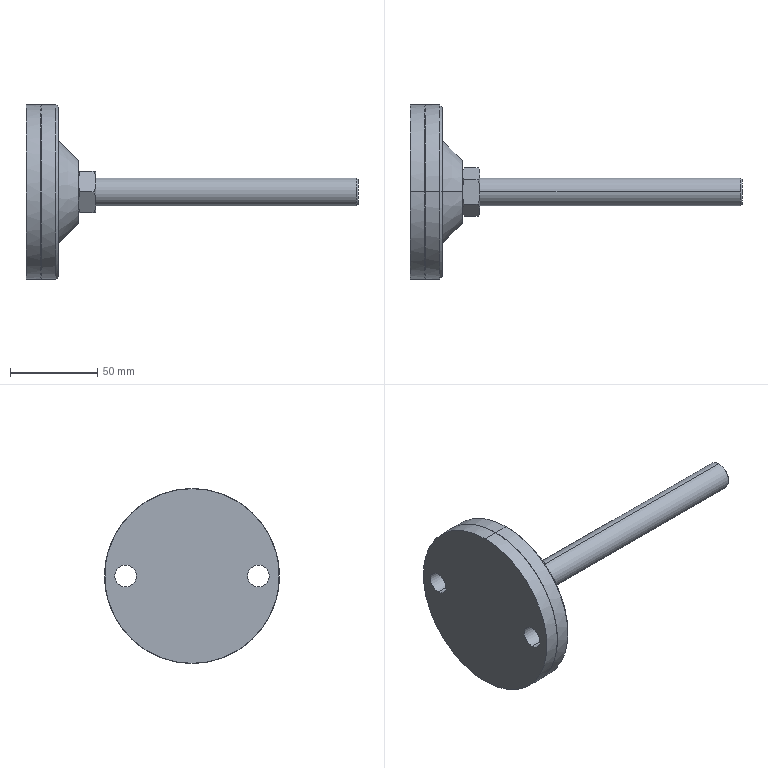Part | STEP file | C-CPVCH16-150 | 1 solid | 34 faces | box 190 x 100 x 100 mm | volume 196270 mm3 | plane 12 | cylinder 10 | cone 8 | spline 4 | commonest cylinder face diameters 12.5 x4 100 x4 16 x2
STEP:
#1=CARTESIAN_POINT('',(31.,-6.928,12.));
#2=VERTEX_POINT('',#1);
#3=CARTESIAN_POINT('',(30.133,0.,12.));
#4=VERTEX_POINT('',#3);
#5=CARTESIAN_POINT('',(31.,-6.928,12.));
#6=CARTESIAN_POINT('',(30.792,-6.375,12.));
#7=CARTESIAN_POINT('',(30.643,-5.81,12.));
#8=CARTESIAN_POINT('',(30.414,-4.667,12.));
#9=CARTESIAN_POINT('',(30.335,-4.089,12.));
#10=CARTESIAN_POINT('',(30.221,-2.923,12.));
#11=CARTESIAN_POINT('',(30.186,-2.337,12.));
#12=CARTESIAN_POINT('',(30.142,-1.168,12.));
#13=CARTESIAN_POINT('',(30.133,-0.5839,12.));
#14=CARTESIAN_POINT('',(30.133,0.,12.));
#15=B_SPLINE_CURVE_WITH_KNOTS('',3,(#5,#6,#7,#8,#9,#10,#11,#12,#13,#14),.UNSPECIFIED.,.F.,.F.,(4,2,2,2,4),(0.,0.001749,0.003497,0.005246,0.006994),.UNSPECIFIED.);
#16=EDGE_CURVE('',#2,#4,#15,.T.);
#17=ORIENTED_EDGE('',*,*,#16,.T.);
#18=CARTESIAN_POINT('',(30.,0.,10.856));
#19=VERTEX_POINT('',#18);
#20=CARTESIAN_POINT('',(35.,0.,10.856));
#21=DIRECTION('',(0.,-1.,0.));
#22=DIRECTION('',(0.,0.,1.));
#23=AXIS2_PLACEMENT_3D('',#20,#21,#22);
#24=CIRCLE('',#23,5.);
#25=EDGE_CURVE('',#4,#19,#24,.T.);
#26=ORIENTED_EDGE('',*,*,#25,.T.);
#27=CARTESIAN_POINT('',(30.,0.,-10.856));
#28=VERTEX_POINT('',#27);
#29=CARTESIAN_POINT('',(30.,0.,10.856));
#30=CARTESIAN_POINT('',(30.,-21.713,10.856));
#31=CARTESIAN_POINT('',(30.,-21.713,-10.856));
#32=CARTESIAN_POINT('',(30.,0.,-10.856));
#33=(BOUNDED_CURVE()B_SPLINE_CURVE(3,(#29,#30,#31,#32),.UNSPECIFIED.,.F.,.T.)B_SPLINE_CURVE_WITH_KNOTS((4,4),(0.5,1.),.UNSPECIFIED.)CURVE()GEOMETRIC_REPRESENTATION_ITEM()RATIONAL_B_SPLINE_CURVE((1.,0.3333,0.3333,1.))REPRESENTATION_ITEM(''));
#34=EDGE_CURVE('',#19,#28,#33,.T.);
#35=ORIENTED_EDGE('',*,*,#34,.T.);
#36=CARTESIAN_POINT('',(30.133,0.,-12.));
#37=VERTEX_POINT('',#36);
#38=CARTESIAN_POINT('',(35.,0.,-10.856));
#39=DIRECTION('',(0.,1.,0.));
#40=DIRECTION('',(0.,0.,-1.));
#41=AXIS2_PLACEMENT_3D('',#38,#39,#40);
#42=CIRCLE('',#41,5.);
#43=EDGE_CURVE('',#37,#28,#42,.T.);
#44=ORIENTED_EDGE('',*,*,#43,.F.);
#45=CARTESIAN_POINT('',(31.,-6.928,-12.));
#46=VERTEX_POINT('',#45);
#47=CARTESIAN_POINT('',(30.133,0.,-12.));
#48=CARTESIAN_POINT('',(30.133,-0.583,-12.));
#49=CARTESIAN_POINT('',(30.142,-1.166,-12.));
#50=CARTESIAN_POINT('',(30.186,-2.33,-12.));
#51=CARTESIAN_POINT('',(30.221,-2.912,-12.));
#52=CARTESIAN_POINT('',(30.334,-4.075,-12.));
#53=CARTESIAN_POINT('',(30.413,-4.659,-12.));
#54=CARTESIAN_POINT('',(30.643,-5.81,-12.));
#55=CARTESIAN_POINT('',(30.793,-6.376,-12.));
#56=CARTESIAN_POINT('',(31.,-6.928,-12.));
#57=B_SPLINE_CURVE_WITH_KNOTS('',3,(#47,#48,#49,#50,#51,#52,#53,#54,#55,#56),.UNSPECIFIED.,.F.,.F.,(4,2,2,2,4),(0.006994,0.00874,0.01049,0.01223,0.01398),.UNSPECIFIED.);
#58=EDGE_CURVE('',#37,#46,#57,.T.);
#59=ORIENTED_EDGE('',*,*,#58,.T.);
#60=CARTESIAN_POINT('',(31.,-13.856,0.));
#61=VERTEX_POINT('',#60);
#62=CARTESIAN_POINT('',(31.,-6.928,-12.));
#63=CARTESIAN_POINT('',(30.793,-7.205,-11.521));
#64=CARTESIAN_POINT('',(30.643,-7.487,-11.032));
#65=CARTESIAN_POINT('',(30.414,-8.058,-10.043));
#66=CARTESIAN_POINT('',(30.336,-8.347,-9.543));
#67=CARTESIAN_POINT('',(30.222,-8.929,-8.534));
#68=CARTESIAN_POINT('',(30.187,-9.222,-8.027));
#69=CARTESIAN_POINT('',(30.142,-9.806,-7.015));
#70=CARTESIAN_POINT('',(30.133,-10.098,-6.51));
#71=CARTESIAN_POINT('',(30.132,-10.681,-5.499));
#72=CARTESIAN_POINT('',(30.142,-10.973,-4.994));
#73=CARTESIAN_POINT('',(30.186,-11.556,-3.985));
#74=CARTESIAN_POINT('',(30.221,-11.847,-3.48));
#75=CARTESIAN_POINT('',(30.333,-12.429,-2.473));
#76=CARTESIAN_POINT('',(30.412,-12.721,-1.967));
#77=CARTESIAN_POINT('',(30.642,-13.297,-0.9692));
#78=CARTESIAN_POINT('',(30.793,-13.58,-0.4783));
#79=CARTESIAN_POINT('',(31.,-13.856,0.));
#80=B_SPLINE_CURVE_WITH_KNOTS('',3,(#62,#63,#64,#65,#66,#67,#68,#69,#70,#71,#72,#73,#74,#75,#76,#77,#78,#79),.UNSPECIFIED.,.F.,.F.,(4,2,2,2,2,2,2,2,4),(0.,0.001747,0.003494,0.005242,0.006989,0.008736,0.01048,0.01223,0.01398),.UNSPECIFIED.);
#81=EDGE_CURVE('',#46,#61,#80,.T.);
#82=ORIENTED_EDGE('',*,*,#81,.T.);
#83=CARTESIAN_POINT('',(31.,-13.856,0.));
#84=CARTESIAN_POINT('',(30.793,-13.58,0.4789));
#85=CARTESIAN_POINT('',(30.643,-13.298,0.9675));
#86=CARTESIAN_POINT('',(30.414,-12.727,1.957));
#87=CARTESIAN_POINT('',(30.336,-12.438,2.457));
#88=CARTESIAN_POINT('',(30.222,-11.855,3.466));
#89=CARTESIAN_POINT('',(30.187,-11.563,3.973));
#90=CARTESIAN_POINT('',(30.142,-10.979,4.985));
#91=CARTESIAN_POINT('',(30.133,-10.687,5.49));
#92=CARTESIAN_POINT('',(30.132,-10.103,6.501));
#93=CARTESIAN_POINT('',(30.142,-9.812,7.006));
#94=CARTESIAN_POINT('',(30.186,-9.229,8.015));
#95=CARTESIAN_POINT('',(30.221,-8.938,8.52));
#96=CARTESIAN_POINT('',(30.333,-8.356,9.527));
#97=CARTESIAN_POINT('',(30.412,-8.064,10.033));
#98=CARTESIAN_POINT('',(30.642,-7.488,11.031));
#99=CARTESIAN_POINT('',(30.793,-7.204,11.522));
#100=CARTESIAN_POINT('',(31.,-6.928,12.));
#101=B_SPLINE_CURVE_WITH_KNOTS('',3,(#83,#84,#85,#86,#87,#88,#89,#90,#91,#92,#93,#94,#95,#96,#97,#98,#99,#100),.UNSPECIFIED.,.F.,.F.,(4,2,2,2,2,2,2,2,4),(0.,0.001747,0.003494,0.005242,0.006989,0.008736,0.01048,0.01223,0.01398),.UNSPECIFIED.);
#102=EDGE_CURVE('',#61,#2,#101,.T.);
#103=ORIENTED_EDGE('',*,*,#102,.T.);
#104=EDGE_LOOP('',(#17,#26,#35,#44,#59,#82,#103));
#105=FACE_OUTER_BOUND('',#104,.T.);
#106=CARTESIAN_POINT('',(31.012,0.,13.872));
#107=CARTESIAN_POINT('',(31.012,-27.744,13.872));
#108=CARTESIAN_POINT('',(31.012,-27.744,-13.872));
#109=CARTESIAN_POINT('',(31.012,0.,-13.872));
#110=CARTESIAN_POINT('',(30.349,0.,12.996));
#111=CARTESIAN_POINT('',(30.349,-25.992,12.996));
#112=CARTESIAN_POINT('',(30.349,-25.992,-12.996));
#113=CARTESIAN_POINT('',(30.349,0.,-12.996));
#114=CARTESIAN_POINT('',(30.,0.,11.955));
#115=CARTESIAN_POINT('',(30.,-23.909,11.955));
#116=CARTESIAN_POINT('',(30.,-23.909,-11.955));
#117=CARTESIAN_POINT('',(30.,0.,-11.955));
#118=CARTESIAN_POINT('',(30.,0.,10.856));
#119=CARTESIAN_POINT('',(30.,-21.713,10.856));
#120=CARTESIAN_POINT('',(30.,-21.713,-10.856));
#121=CARTESIAN_POINT('',(30.,0.,-10.856));
#122=(BOUNDED_SURFACE()B_SPLINE_SURFACE(3,3,((#106,#107,#108,#109),(#110,#111,#112,#113),(#114,#115,#116,#117),(#118,#119,#120,#121)),.UNSPECIFIED.,.F.,.F.,.F.)B_SPLINE_SURFACE_WITH_KNOTS((4,4),(4,4),(0.,1.),(0.,1.),.UNSPECIFIED.)GEOMETRIC_REPRESENTATION_ITEM()RATIONAL_B_SPLINE_SURFACE(((1.,0.3333,0.3333,1.),(0.9654,0.3218,0.3218,0.9654),(0.9654,0.3218,0.3218,0.9654),(1.,0.3333,0.3333,1.)))REPRESENTATION_ITEM('')SURFACE());
#123=ADVANCED_FACE('',(#105),#122,.T.);
#124=CARTESIAN_POINT('',(40.,0.,-10.856));
#125=VERTEX_POINT('',#124);
#126=CARTESIAN_POINT('',(40.,0.,10.856));
#127=VERTEX_POINT('',#126);
#128=CARTESIAN_POINT('',(40.,0.,-10.856));
#129=CARTESIAN_POINT('',(40.,-21.713,-10.856));
#130=CARTESIAN_POINT('',(40.,-21.713,10.856));
#131=CARTESIAN_POINT('',(40.,0.,10.856));
#132=(BOUNDED_CURVE()B_SPLINE_CURVE(3,(#128,#129,#130,#131),.UNSPECIFIED.,.F.,.F.)B_SPLINE_CURVE_WITH_KNOTS((4,4),(0.,0.5),.UNSPECIFIED.)CURVE()GEOMETRIC_REPRESENTATION_ITEM()RATIONAL_B_SPLINE_CURVE((1.,0.3333,0.3333,1.))REPRESENTATION_ITEM(''));
#133=EDGE_CURVE('',#125,#127,#132,.T.);
#134=ORIENTED_EDGE('',*,*,#133,.T.);
#135=CARTESIAN_POINT('',(39.867,0.,12.));
#136=VERTEX_POINT('',#135);
#137=CARTESIAN_POINT('',(35.,0.,10.856));
#138=DIRECTION('',(0.,-1.,0.));
#139=DIRECTION('',(0.,0.,1.));
#140=AXIS2_PLACEMENT_3D('',#137,#138,#139);
#141=CIRCLE('',#140,5.);
#142=EDGE_CURVE('',#127,#136,#141,.T.);
#143=ORIENTED_EDGE('',*,*,#142,.T.);
#144=CARTESIAN_POINT('',(39.,-6.928,12.));
#145=VERTEX_POINT('',#144);
#146=CARTESIAN_POINT('',(39.867,0.,12.));
#147=CARTESIAN_POINT('',(39.867,-0.583,12.));
#148=CARTESIAN_POINT('',(39.858,-1.166,12.));
#149=CARTESIAN_POINT('',(39.814,-2.33,12.));
#150=CARTESIAN_POINT('',(39.779,-2.912,12.));
#151=CARTESIAN_POINT('',(39.666,-4.075,12.));
#152=CARTESIAN_POINT('',(39.587,-4.659,12.));
#153=CARTESIAN_POINT('',(39.357,-5.81,12.));
#154=CARTESIAN_POINT('',(39.207,-6.376,12.));
#155=CARTESIAN_POINT('',(39.,-6.928,12.));
#156=B_SPLINE_CURVE_WITH_KNOTS('',3,(#146,#147,#148,#149,#150,#151,#152,#153,#154,#155),.UNSPECIFIED.,.F.,.F.,(4,2,2,2,4),(0.006994,0.00874,0.01049,0.01223,0.01398),.UNSPECIFIED.);
#157=EDGE_CURVE('',#136,#145,#156,.T.);
#158=ORIENTED_EDGE('',*,*,#157,.T.);
#159=CARTESIAN_POINT('',(39.,-13.856,0.));
#160=VERTEX_POINT('',#159);
#161=CARTESIAN_POINT('',(39.,-6.928,12.));
#162=CARTESIAN_POINT('',(39.207,-7.205,11.521));
#163=CARTESIAN_POINT('',(39.357,-7.487,11.032));
#164=CARTESIAN_POINT('',(39.586,-8.058,10.043));
#165=CARTESIAN_POINT('',(39.664,-8.347,9.543));
#166=CARTESIAN_POINT('',(39.778,-8.929,8.534));
#167=CARTESIAN_POINT('',(39.813,-9.222,8.027));
#168=CARTESIAN_POINT('',(39.858,-9.806,7.015));
#169=CARTESIAN_POINT('',(39.867,-10.098,6.51));
#170=CARTESIAN_POINT('',(39.868,-10.681,5.499));
#171=CARTESIAN_POINT('',(39.858,-10.973,4.994));
#172=CARTESIAN_POINT('',(39.814,-11.556,3.985));
#173=CARTESIAN_POINT('',(39.779,-11.847,3.48));
#174=CARTESIAN_POINT('',(39.667,-12.429,2.473));
#175=CARTESIAN_POINT('',(39.588,-12.721,1.967));
#176=CARTESIAN_POINT('',(39.358,-13.297,0.9692));
#177=CARTESIAN_POINT('',(39.207,-13.58,0.4783));
#178=CARTESIAN_POINT('',(39.,-13.856,0.));
#179=B_SPLINE_CURVE_WITH_KNOTS('',3,(#161,#162,#163,#164,#165,#166,#167,#168,#169,#170,#171,#172,#173,#174,#175,#176,#177,#178),.UNSPECIFIED.,.F.,.F.,(4,2,2,2,2,2,2,2,4),(0.,0.001747,0.003494,0.005242,0.006989,0.008736,0.01048,0.01223,0.01398),.UNSPECIFIED.);
#180=EDGE_CURVE('',#145,#160,#179,.T.);
#181=ORIENTED_EDGE('',*,*,#180,.T.);
#182=CARTESIAN_POINT('',(39.,-6.928,-12.));
#183=VERTEX_POINT('',#182);
#184=CARTESIAN_POINT('',(39.,-13.856,0.));
#185=CARTESIAN_POINT('',(39.207,-13.58,-0.4789));
#186=CARTESIAN_POINT('',(39.357,-13.298,-0.9675));
#187=CARTESIAN_POINT('',(39.586,-12.727,-1.957));
#188=CARTESIAN_POINT('',(39.664,-12.438,-2.457));
#189=CARTESIAN_POINT('',(39.778,-11.855,-3.466));
#190=CARTESIAN_POINT('',(39.813,-11.563,-3.973));
#191=CARTESIAN_POINT('',(39.858,-10.979,-4.985));
#192=CARTESIAN_POINT('',(39.867,-10.687,-5.49));
#193=CARTESIAN_POINT('',(39.868,-10.103,-6.501));
#194=CARTESIAN_POINT('',(39.858,-9.812,-7.006));
#195=CARTESIAN_POINT('',(39.814,-9.229,-8.015));
#196=CARTESIAN_POINT('',(39.779,-8.938,-8.52));
#197=CARTESIAN_POINT('',(39.667,-8.356,-9.527));
#198=CARTESIAN_POINT('',(39.588,-8.064,-10.033));
#199=CARTESIAN_POINT('',(39.358,-7.488,-11.031));
#200=CARTESIAN_POINT('',(39.207,-7.204,-11.522));
#201=CARTESIAN_POINT('',(39.,-6.928,-12.));
#202=B_SPLINE_CURVE_WITH_KNOTS('',3,(#184,#185,#186,#187,#188,#189,#190,#191,#192,#193,#194,#195,#196,#197,#198,#199,#200,#201),.UNSPECIFIED.,.F.,.F.,(4,2,2,2,2,2,2,2,4),(0.,0.001747,0.003494,0.005242,0.006989,0.008736,0.01048,0.01223,0.01398),.UNSPECIFIED.);
#203=EDGE_CURVE('',#160,#183,#202,.T.);
#204=ORIENTED_EDGE('',*,*,#203,.T.);
#205=CARTESIAN_POINT('',(39.867,0.,-12.));
#206=VERTEX_POINT('',#205);
#207=CARTESIAN_POINT('',(39.,-6.928,-12.));
#208=CARTESIAN_POINT('',(39.208,-6.375,-12.));
#209=CARTESIAN_POINT('',(39.357,-5.81,-12.));
#210=CARTESIAN_POINT('',(39.586,-4.667,-12.));
#211=CARTESIAN_POINT('',(39.665,-4.089,-12.));
#212=CARTESIAN_POINT('',(39.779,-2.923,-12.));
#213=CARTESIAN_POINT('',(39.814,-2.337,-12.));
#214=CARTESIAN_POINT('',(39.858,-1.168,-12.));
#215=CARTESIAN_POINT('',(39.867,-0.5839,-12.));
#216=CARTESIAN_POINT('',(39.867,0.,-12.));
#217=B_SPLINE_CURVE_WITH_KNOTS('',3,(#207,#208,#209,#210,#211,#212,#213,#214,#215,#216),.UNSPECIFIED.,.F.,.F.,(4,2,2,2,4),(0.,0.001749,0.003497,0.005246,0.006994),.UNSPECIFIED.);
#218=EDGE_CURVE('',#183,#206,#217,.T.);
#219=ORIENTED_EDGE('',*,*,#218,.T.);
#220=CARTESIAN_POINT('',(35.,0.,-10.856));
#221=DIRECTION('',(0.,1.,0.));
#222=DIRECTION('',(0.,0.,-1.));
#223=AXIS2_PLACEMENT_3D('',#220,#221,#222);
#224=CIRCLE('',#223,5.);
#225=EDGE_CURVE('',#125,#206,#224,.T.);
#226=ORIENTED_EDGE('',*,*,#225,.F.);
#227=EDGE_LOOP('',(#134,#143,#158,#181,#204,#219,#226));
#228=FACE_OUTER_BOUND('',#227,.T.);
#229=CARTESIAN_POINT('',(40.,0.,10.856));
#230=CARTESIAN_POINT('',(40.,-21.713,10.856));
#231=CARTESIAN_POINT('',(40.,-21.713,-10.856));
#232=CARTESIAN_POINT('',(40.,0.,-10.856));
#233=CARTESIAN_POINT('',(40.,0.,11.955));
#234=CARTESIAN_POINT('',(40.,-23.909,11.955));
#235=CARTESIAN_POINT('',(40.,-23.909,-11.955));
#236=CARTESIAN_POINT('',(40.,0.,-11.955));
#237=CARTESIAN_POINT('',(39.651,0.,12.996));
#238=CARTESIAN_POINT('',(39.651,-25.992,12.996));
#239=CARTESIAN_POINT('',(39.651,-25.992,-12.996));
#240=CARTESIAN_POINT('',(39.651,0.,-12.996));
#241=CARTESIAN_POINT('',(38.988,0.,13.872));
#242=CARTESIAN_POINT('',(38.988,-27.744,13.872));
#243=CARTESIAN_POINT('',(38.988,-27.744,-13.872));
#244=CARTESIAN_POINT('',(38.988,0.,-13.872));
#245=(BOUNDED_SURFACE()B_SPLINE_SURFACE(3,3,((#229,#230,#231,#232),(#233,#234,#235,#236),(#237,#238,#239,#240),(#241,#242,#243,#244)),.UNSPECIFIED.,.F.,.F.,.F.)B_SPLINE_SURFACE_WITH_KNOTS((4,4),(4,4),(0.,1.),(0.,1.),.UNSPECIFIED.)GEOMETRIC_REPRESENTATION_ITEM()RATIONAL_B_SPLINE_SURFACE(((1.,0.3333,0.3333,1.),(0.9654,0.3218,0.3218,0.9654),(0.9654,0.3218,0.3218,0.9654),(1.,0.3333,0.3333,1.)))REPRESENTATION_ITEM('')SURFACE());
#246=ADVANCED_FACE('',(#228),#245,.T.);
#247=CARTESIAN_POINT('',(18.5,-38.,-6.25));
#248=VERTEX_POINT('',#247);
#249=CARTESIAN_POINT('',(18.5,-38.,6.25));
#250=VERTEX_POINT('',#249);
#251=CARTESIAN_POINT('',(18.5,-38.,0.));
#252=DIRECTION('',(-1.,0.,0.));
#253=DIRECTION('',(0.,0.,1.));
#254=AXIS2_PLACEMENT_3D('',#251,#252,#253);
#255=CIRCLE('',#254,6.25);
#256=EDGE_CURVE('',#248,#250,#255,.T.);
#257=ORIENTED_EDGE('',*,*,#256,.F.);
#258=CARTESIAN_POINT('',(0.,-38.,-6.25));
#259=VERTEX_POINT('',#258);
#260=CARTESIAN_POINT('',(18.5,-38.,-6.25));
#261=DIRECTION('',(-1.,0.,0.));
#262=VECTOR('',#261,1000.);
#263=LINE('',#260,#262);
#264=EDGE_CURVE('',#248,#259,#263,.T.);
#265=ORIENTED_EDGE('',*,*,#264,.T.);
#266=CARTESIAN_POINT('',(0.,-38.,6.25));
#267=VERTEX_POINT('',#266);
#268=CARTESIAN_POINT('',(0.,-38.,0.));
#269=DIRECTION('',(-1.,0.,0.));
#270=DIRECTION('',(0.,0.,1.));
#271=AXIS2_PLACEMENT_3D('',#268,#269,#270);
#272=CIRCLE('',#271,6.25);
#273=EDGE_CURVE('',#259,#267,#272,.T.);
#274=ORIENTED_EDGE('',*,*,#273,.T.);
#275=CARTESIAN_POINT('',(18.5,-38.,6.25));
#276=DIRECTION('',(-1.,0.,0.));
#277=VECTOR('',#276,1000.);
#278=LINE('',#275,#277);
#279=EDGE_CURVE('',#250,#267,#278,.T.);
#280=ORIENTED_EDGE('',*,*,#279,.F.);
#281=EDGE_LOOP('',(#257,#265,#274,#280));
#282=FACE_OUTER_BOUND('',#281,.T.);
#283=CARTESIAN_POINT('',(18.5,-38.,0.));
#284=DIRECTION('',(-1.,0.,0.));
#285=DIRECTION('',(0.,0.,1.));
#286=AXIS2_PLACEMENT_3D('',#283,#284,#285);
#287=CYLINDRICAL_SURFACE('',#286,6.25);
#288=ADVANCED_FACE('',(#282),#287,.F.);
#289=CARTESIAN_POINT('',(18.5,38.,-6.25));
#290=VERTEX_POINT('',#289);
#291=CARTESIAN_POINT('',(18.5,38.,6.25));
#292=VERTEX_POINT('',#291);
#293=CARTESIAN_POINT('',(18.5,38.,0.));
#294=DIRECTION('',(-1.,0.,0.));
#295=DIRECTION('',(0.,0.,1.));
#296=AXIS2_PLACEMENT_3D('',#293,#294,#295);
#297=CIRCLE('',#296,6.25);
#298=EDGE_CURVE('',#290,#292,#297,.T.);
#299=ORIENTED_EDGE('',*,*,#298,.F.);
#300=CARTESIAN_POINT('',(0.,38.,-6.25));
#301=VERTEX_POINT('',#300);
#302=CARTESIAN_POINT('',(18.5,38.,-6.25));
#303=DIRECTION('',(-1.,0.,0.));
#304=VECTOR('',#303,1000.);
#305=LINE('',#302,#304);
#306=EDGE_CURVE('',#290,#301,#305,.T.);
#307=ORIENTED_EDGE('',*,*,#306,.T.);
#308=CARTESIAN_POINT('',(0.,38.,6.25));
#309=VERTEX_POINT('',#308);
#310=CARTESIAN_POINT('',(0.,38.,0.));
#311=DIRECTION('',(-1.,0.,0.));
#312=DIRECTION('',(0.,0.,1.));
#313=AXIS2_PLACEMENT_3D('',#310,#311,#312);
#314=CIRCLE('',#313,6.25);
#315=EDGE_CURVE('',#301,#309,#314,.T.);
#316=ORIENTED_EDGE('',*,*,#315,.T.);
#317=CARTESIAN_POINT('',(18.5,38.,6.25));
#318=DIRECTION('',(-1.,0.,0.));
#319=VECTOR('',#318,1000.);
#320=LINE('',#317,#319);
#321=EDGE_CURVE('',#292,#309,#320,.T.);
#322=ORIENTED_EDGE('',*,*,#321,.F.);
#323=EDGE_LOOP('',(#299,#307,#316,#322));
#324=FACE_OUTER_BOUND('',#323,.T.);
#325=CARTESIAN_POINT('',(18.5,38.,0.));
#326=DIRECTION('',(-1.,0.,0.));
#327=DIRECTION('',(0.,0.,1.));
#328=AXIS2_PLACEMENT_3D('',#325,#326,#327);
#329=CYLINDRICAL_SURFACE('',#328,6.25);
#330=ADVANCED_FACE('',(#324),#329,.F.);
#331=CARTESIAN_POINT('',(8.5,0.,50.));
#332=VERTEX_POINT('',#331);
#333=CARTESIAN_POINT('',(8.5,0.,-50.));
#334=VERTEX_POINT('',#333);
#335=CARTESIAN_POINT('',(8.5,0.,0.));
#336=DIRECTION('',(-1.,0.,0.));
#337=DIRECTION('',(0.,0.,1.));
#338=AXIS2_PLACEMENT_3D('',#335,#336,#337);
#339=CIRCLE('',#338,50.);
#340=EDGE_CURVE('',#332,#334,#339,.T.);
#341=ORIENTED_EDGE('',*,*,#340,.T.);
#342=CARTESIAN_POINT('',(0.,0.,-50.));
#343=VERTEX_POINT('',#342);
#344=CARTESIAN_POINT('',(190.,0.,-50.));
#345=DIRECTION('',(-1.,0.,0.));
#346=VECTOR('',#345,1000.);
#347=LINE('',#344,#346);
#348=EDGE_CURVE('',#334,#343,#347,.T.);
#349=ORIENTED_EDGE('',*,*,#348,.T.);
#350=CARTESIAN_POINT('',(0.,0.,50.));
#351=VERTEX_POINT('',#350);
#352=CARTESIAN_POINT('',(0.,0.,0.));
#353=DIRECTION('',(1.,0.,0.));
#354=DIRECTION('',(0.,0.,1.));
#355=AXIS2_PLACEMENT_3D('',#352,#353,#354);
#356=CIRCLE('',#355,50.);
#357=EDGE_CURVE('',#343,#351,#356,.T.);
#358=ORIENTED_EDGE('',*,*,#357,.T.);
#359=CARTESIAN_POINT('',(190.,0.,50.));
#360=DIRECTION('',(-1.,0.,0.));
#361=VECTOR('',#360,1000.);
#362=LINE('',#359,#361);
#363=EDGE_CURVE('',#332,#351,#362,.T.);
#364=ORIENTED_EDGE('',*,*,#363,.F.);
#365=EDGE_LOOP('',(#341,#349,#358,#364));
#366=FACE_OUTER_BOUND('',#365,.T.);
#367=CARTESIAN_POINT('',(190.,0.,0.));
#368=DIRECTION('',(-1.,0.,0.));
#369=DIRECTION('',(0.,0.,1.));
#370=AXIS2_PLACEMENT_3D('',#367,#368,#369);
#371=CYLINDRICAL_SURFACE('',#370,50.);
#372=ADVANCED_FACE('',(#366),#371,.T.);
#373=CARTESIAN_POINT('',(18.5,0.,48.5));
#374=VERTEX_POINT('',#373);
#375=CARTESIAN_POINT('',(18.5,0.,-48.5));
#376=VERTEX_POINT('',#375);
#377=CARTESIAN_POINT('',(18.5,0.,0.));
#378=DIRECTION('',(-1.,0.,0.));
#379=DIRECTION('',(0.,0.,1.));
#380=AXIS2_PLACEMENT_3D('',#377,#378,#379);
#381=CIRCLE('',#380,48.5);
#382=EDGE_CURVE('',#374,#376,#381,.T.);
#383=ORIENTED_EDGE('',*,*,#382,.T.);
#384=CARTESIAN_POINT('',(17.,0.,-50.));
#385=VERTEX_POINT('',#384);
#386=CARTESIAN_POINT('',(17.,0.,-50.));
#387=DIRECTION('',(-0.7071,0.,-0.7071));
#388=VECTOR('',#387,1000.);
#389=LINE('',#386,#388);
#390=EDGE_CURVE('',#376,#385,#389,.T.);
#391=ORIENTED_EDGE('',*,*,#390,.T.);
#392=CARTESIAN_POINT('',(17.,0.,50.));
#393=VERTEX_POINT('',#392);
#394=CARTESIAN_POINT('',(17.,0.,0.));
#395=DIRECTION('',(1.,0.,0.));
#396=DIRECTION('',(0.,0.,1.));
#397=AXIS2_PLACEMENT_3D('',#394,#395,#396);
#398=CIRCLE('',#397,50.);
#399=EDGE_CURVE('',#385,#393,#398,.T.);
#400=ORIENTED_EDGE('',*,*,#399,.T.);
#401=CARTESIAN_POINT('',(17.,0.,50.));
#402=DIRECTION('',(-0.7071,0.,0.7071));
#403=VECTOR('',#402,1000.);
#404=LINE('',#401,#403);
#405=EDGE_CURVE('',#374,#393,#404,.T.);
#406=ORIENTED_EDGE('',*,*,#405,.F.);
#407=EDGE_LOOP('',(#383,#391,#400,#406));
#408=FACE_OUTER_BOUND('',#407,.T.);
#409=CARTESIAN_POINT('',(17.,0.,0.));
#410=DIRECTION('',(-1.,0.,0.));
#411=DIRECTION('',(0.,0.,1.));
#412=AXIS2_PLACEMENT_3D('',#409,#410,#411);
#413=CONICAL_SURFACE('',#412,50.,0.7854);
#414=ADVANCED_FACE('',(#408),#413,.T.);
#415=CARTESIAN_POINT('',(30.,0.,18.));
#416=VERTEX_POINT('',#415);
#417=CARTESIAN_POINT('',(30.,0.,-18.));
#418=VERTEX_POINT('',#417);
#419=CARTESIAN_POINT('',(30.,0.,0.));
#420=DIRECTION('',(-1.,0.,0.));
#421=DIRECTION('',(0.,0.,1.));
#422=AXIS2_PLACEMENT_3D('',#419,#420,#421);
#423=CIRCLE('',#422,18.);
#424=EDGE_CURVE('',#416,#418,#423,.T.);
#425=ORIENTED_EDGE('',*,*,#424,.T.);
#426=CARTESIAN_POINT('',(18.5,0.,-29.5));
#427=VERTEX_POINT('',#426);
#428=CARTESIAN_POINT('',(18.5,0.,-29.5));
#429=DIRECTION('',(-0.7071,0.,-0.7071));
#430=VECTOR('',#429,1000.);
#431=LINE('',#428,#430);
#432=EDGE_CURVE('',#418,#427,#431,.T.);
#433=ORIENTED_EDGE('',*,*,#432,.T.);
#434=CARTESIAN_POINT('',(18.5,0.,29.5));
#435=VERTEX_POINT('',#434);
#436=CARTESIAN_POINT('',(18.5,0.,0.));
#437=DIRECTION('',(1.,0.,0.));
#438=DIRECTION('',(0.,0.,1.));
#439=AXIS2_PLACEMENT_3D('',#436,#437,#438);
#440=CIRCLE('',#439,29.5);
#441=EDGE_CURVE('',#427,#435,#440,.T.);
#442=ORIENTED_EDGE('',*,*,#441,.T.);
#443=CARTESIAN_POINT('',(18.5,0.,29.5));
#444=DIRECTION('',(-0.7071,0.,0.7071));
#445=VECTOR('',#444,1000.);
#446=LINE('',#443,#445);
#447=EDGE_CURVE('',#416,#435,#446,.T.);
#448=ORIENTED_EDGE('',*,*,#447,.F.);
#449=EDGE_LOOP('',(#425,#433,#442,#448));
#450=FACE_OUTER_BOUND('',#449,.T.);
#451=CARTESIAN_POINT('',(18.5,0.,0.));
#452=DIRECTION('',(-1.,0.,0.));
#453=DIRECTION('',(0.,0.,1.));
#454=AXIS2_PLACEMENT_3D('',#451,#452,#453);
#455=CONICAL_SURFACE('',#454,29.5,0.7854);
#456=ADVANCED_FACE('',(#450),#455,.T.);
#457=CARTESIAN_POINT('',(8.5,49.9,0.));
#458=VERTEX_POINT('',#457);
#459=CARTESIAN_POINT('',(8.5,-49.9,0.));
#460=VERTEX_POINT('',#459);
#461=CARTESIAN_POINT('',(8.5,0.,0.));
#462=DIRECTION('',(1.,0.,0.));
#463=DIRECTION('',(0.,1.,0.));
#464=AXIS2_PLACEMENT_3D('',#461,#462,#463);
#465=CIRCLE('',#464,49.9);
#466=EDGE_CURVE('',#458,#460,#465,.T.);
#467=ORIENTED_EDGE('',*,*,#466,.T.);
#468=CARTESIAN_POINT('',(8.6,-50.,0.));
#469=VERTEX_POINT('',#468);
#470=CARTESIAN_POINT('',(8.6,-50.,0.));
#471=DIRECTION('',(0.7071,-0.7071,0.));
#472=VECTOR('',#471,1000.);
#473=LINE('',#470,#472);
#474=EDGE_CURVE('',#460,#469,#473,.T.);
#475=ORIENTED_EDGE('',*,*,#474,.T.);
#476=CARTESIAN_POINT('',(8.6,0.,50.));
#477=VERTEX_POINT('',#476);
#478=CARTESIAN_POINT('',(8.6,0.,0.));
#479=DIRECTION('',(-1.,0.,0.));
#480=DIRECTION('',(0.,0.,-1.));
#481=AXIS2_PLACEMENT_3D('',#478,#479,#480);
#482=CIRCLE('',#481,50.);
#483=EDGE_CURVE('',#469,#477,#482,.T.);
#484=ORIENTED_EDGE('',*,*,#483,.T.);
#485=CARTESIAN_POINT('',(8.6,50.,0.));
#486=VERTEX_POINT('',#485);
#487=CARTESIAN_POINT('',(8.6,0.,0.));
#488=DIRECTION('',(-1.,0.,0.));
#489=DIRECTION('',(0.,0.,-1.));
#490=AXIS2_PLACEMENT_3D('',#487,#488,#489);
#491=CIRCLE('',#490,50.);
#492=EDGE_CURVE('',#477,#486,#491,.T.);
#493=ORIENTED_EDGE('',*,*,#492,.T.);
#494=CARTESIAN_POINT('',(8.6,50.,0.));
#495=DIRECTION('',(0.7071,0.7071,0.));
#496=VECTOR('',#495,1000.);
#497=LINE('',#494,#496);
#498=EDGE_CURVE('',#458,#486,#497,.T.);
#499=ORIENTED_EDGE('',*,*,#498,.F.);
#500=EDGE_LOOP('',(#467,#475,#484,#493,#499));
#501=FACE_OUTER_BOUND('',#500,.T.);
#502=CARTESIAN_POINT('',(8.6,0.,0.));
#503=DIRECTION('',(1.,0.,0.));
#504=DIRECTION('',(0.,1.,0.));
#505=AXIS2_PLACEMENT_3D('',#502,#503,#504);
#506=CONICAL_SURFACE('',#505,50.,0.7854);
#507=ADVANCED_FACE('',(#501),#506,.T.);
#508=ORIENTED_EDGE('',*,*,#399,.F.);
#509=CARTESIAN_POINT('',(8.6,0.,-50.));
#510=VERTEX_POINT('',#509);
#511=CARTESIAN_POINT('',(190.,0.,-50.));
#512=DIRECTION('',(-1.,0.,0.));
#513=VECTOR('',#512,1000.);
#514=LINE('',#511,#513);
#515=EDGE_CURVE('',#385,#510,#514,.T.);
#516=ORIENTED_EDGE('',*,*,#515,.T.);
#517=CARTESIAN_POINT('',(8.6,0.,0.));
#518=DIRECTION('',(-1.,0.,0.));
#519=DIRECTION('',(0.,0.,-1.));
#520=AXIS2_PLACEMENT_3D('',#517,#518,#519);
#521=CIRCLE('',#520,50.);
#522=EDGE_CURVE('',#486,#510,#521,.T.);
#523=ORIENTED_EDGE('',*,*,#522,.F.);
#524=ORIENTED_EDGE('',*,*,#492,.F.);
#525=CARTESIAN_POINT('',(190.,0.,50.));
#526=DIRECTION('',(-1.,0.,0.));
#527=VECTOR('',#526,1000.);
#528=LINE('',#525,#527);
#529=EDGE_CURVE('',#393,#477,#528,.T.);
#530=ORIENTED_EDGE('',*,*,#529,.F.);
#531=EDGE_LOOP('',(#508,#516,#523,#524,#530));
#532=FACE_OUTER_BOUND('',#531,.T.);
#533=CARTESIAN_POINT('',(190.,0.,0.));
#534=DIRECTION('',(-1.,0.,0.));
#535=DIRECTION('',(0.,0.,1.));
#536=AXIS2_PLACEMENT_3D('',#533,#534,#535);
#537=CYLINDRICAL_SURFACE('',#536,50.);
#538=ADVANCED_FACE('',(#532),#537,.T.);
#539=CARTESIAN_POINT('',(189.,0.,8.));
#540=VERTEX_POINT('',#539);
#541=CARTESIAN_POINT('',(189.,0.,-8.));
#542=VERTEX_POINT('',#541);
#543=CARTESIAN_POINT('',(189.,0.,0.));
#544=DIRECTION('',(-1.,0.,0.));
#545=DIRECTION('',(0.,0.,1.));
#546=AXIS2_PLACEMENT_3D('',#543,#544,#545);
#547=CIRCLE('',#546,8.);
#548=EDGE_CURVE('',#540,#542,#547,.T.);
#549=ORIENTED_EDGE('',*,*,#548,.T.);
#550=CARTESIAN_POINT('',(40.,0.,-8.));
#551=VERTEX_POINT('',#550);
#552=CARTESIAN_POINT('',(190.,0.,-8.));
#553=DIRECTION('',(-1.,0.,0.));
#554=VECTOR('',#553,1000.);
#555=LINE('',#552,#554);
#556=EDGE_CURVE('',#542,#551,#555,.T.);
#557=ORIENTED_EDGE('',*,*,#556,.T.);
#558=CARTESIAN_POINT('',(40.,0.,8.));
#559=VERTEX_POINT('',#558);
#560=CARTESIAN_POINT('',(40.,0.,0.));
#561=DIRECTION('',(1.,0.,0.));
#562=DIRECTION('',(0.,0.,1.));
#563=AXIS2_PLACEMENT_3D('',#560,#561,#562);
#564=CIRCLE('',#563,8.);
#565=EDGE_CURVE('',#551,#559,#564,.T.);
#566=ORIENTED_EDGE('',*,*,#565,.T.);
#567=CARTESIAN_POINT('',(190.,0.,8.));
#568=DIRECTION('',(-1.,0.,0.));
#569=VECTOR('',#568,1000.);
#570=LINE('',#567,#569);
#571=EDGE_CURVE('',#540,#559,#570,.T.);
#572=ORIENTED_EDGE('',*,*,#571,.F.);
#573=EDGE_LOOP('',(#549,#557,#566,#572));
#574=FACE_OUTER_BOUND('',#573,.T.);
#575=CARTESIAN_POINT('',(190.,0.,0.));
#576=DIRECTION('',(-1.,0.,0.));
#577=DIRECTION('',(0.,0.,1.));
#578=AXIS2_PLACEMENT_3D('',#575,#576,#577);
#579=CYLINDRICAL_SURFACE('',#578,8.);
#580=ADVANCED_FACE('',(#574),#579,.T.);
#581=CARTESIAN_POINT('',(190.,0.,7.));
#582=VERTEX_POINT('',#581);
#583=CARTESIAN_POINT('',(190.,0.,-7.));
#584=VERTEX_POINT('',#583);
#585=CARTESIAN_POINT('',(190.,0.,0.));
#586=DIRECTION('',(-1.,0.,0.));
#587=DIRECTION('',(0.,0.,1.));
#588=AXIS2_PLACEMENT_3D('',#585,#586,#587);
#589=CIRCLE('',#588,7.);
#590=EDGE_CURVE('',#582,#584,#589,.T.);
#591=ORIENTED_EDGE('',*,*,#590,.T.);
#592=CARTESIAN_POINT('',(189.,0.,-8.));
#593=DIRECTION('',(-0.7071,0.,-0.7071));
#594=VECTOR('',#593,1000.);
#595=LINE('',#592,#594);
#596=EDGE_CURVE('',#584,#542,#595,.T.);
#597=ORIENTED_EDGE('',*,*,#596,.T.);
#598=ORIENTED_EDGE('',*,*,#548,.F.);
#599=CARTESIAN_POINT('',(189.,0.,8.));
#600=DIRECTION('',(-0.7071,0.,0.7071));
#601=VECTOR('',#600,1000.);
#602=LINE('',#599,#601);
#603=EDGE_CURVE('',#582,#540,#602,.T.);
#604=ORIENTED_EDGE('',*,*,#603,.F.);
#605=EDGE_LOOP('',(#591,#597,#598,#604));
#606=FACE_OUTER_BOUND('',#605,.T.);
#607=CARTESIAN_POINT('',(189.,0.,0.));
#608=DIRECTION('',(-1.,0.,0.));
#609=DIRECTION('',(0.,0.,1.));
#610=AXIS2_PLACEMENT_3D('',#607,#608,#609);
#611=CONICAL_SURFACE('',#610,8.,0.7854);
#612=ADVANCED_FACE('',(#606),#611,.T.);
#613=CARTESIAN_POINT('',(0.,-38.,0.));
#614=DIRECTION('',(-1.,0.,0.));
#615=DIRECTION('',(0.,0.,1.));
#616=AXIS2_PLACEMENT_3D('',#613,#614,#615);
#617=CIRCLE('',#616,6.25);
#618=EDGE_CURVE('',#267,#259,#617,.T.);
#619=ORIENTED_EDGE('',*,*,#618,.F.);
#620=ORIENTED_EDGE('',*,*,#273,.F.);
#621=EDGE_LOOP('',(#619,#620));
#622=FACE_BOUND('',#621,.T.);
#623=CARTESIAN_POINT('',(0.,38.,0.));
#624=DIRECTION('',(-1.,0.,0.));
#625=DIRECTION('',(0.,0.,1.));
#626=AXIS2_PLACEMENT_3D('',#623,#624,#625);
#627=CIRCLE('',#626,6.25);
#628=EDGE_CURVE('',#309,#301,#627,.T.);
#629=ORIENTED_EDGE('',*,*,#628,.F.);
#630=ORIENTED_EDGE('',*,*,#315,.F.);
#631=EDGE_LOOP('',(#629,#630));
#632=FACE_BOUND('',#631,.T.);
#633=CARTESIAN_POINT('',(0.,0.,0.));
#634=DIRECTION('',(1.,0.,0.));
#635=DIRECTION('',(0.,0.,1.));
#636=AXIS2_PLACEMENT_3D('',#633,#634,#635);
#637=CIRCLE('',#636,50.);
#638=EDGE_CURVE('',#351,#343,#637,.T.);
#639=ORIENTED_EDGE('',*,*,#638,.F.);
#640=ORIENTED_EDGE('',*,*,#357,.F.);
#641=EDGE_LOOP('',(#639,#640));
#642=FACE_OUTER_BOUND('',#641,.T.);
#643=CARTESIAN_POINT('',(0.,0.,0.));
#644=DIRECTION('',(1.,0.,0.));
#645=DIRECTION('',(0.,0.,-1.));
#646=AXIS2_PLACEMENT_3D('',#643,#644,#645);
#647=PLANE('',#646);
#648=ADVANCED_FACE('',(#622,#632,#642),#647,.F.);
#649=ORIENTED_EDGE('',*,*,#264,.F.);
#650=CARTESIAN_POINT('',(18.5,-38.,0.));
#651=DIRECTION('',(-1.,0.,0.));
#652=DIRECTION('',(0.,0.,1.));
#653=AXIS2_PLACEMENT_3D('',#650,#651,#652);
#654=CIRCLE('',#653,6.25);
#655=EDGE_CURVE('',#250,#248,#654,.T.);
#656=ORIENTED_EDGE('',*,*,#655,.F.);
#657=ORIENTED_EDGE('',*,*,#279,.T.);
#658=ORIENTED_EDGE('',*,*,#618,.T.);
#659=EDGE_LOOP('',(#649,#656,#657,#658));
#660=FACE_OUTER_BOUND('',#659,.T.);
#661=CARTESIAN_POINT('',(18.5,-38.,0.));
#662=DIRECTION('',(-1.,0.,0.));
#663=DIRECTION('',(0.,0.,1.));
#664=AXIS2_PLACEMENT_3D('',#661,#662,#663);
#665=CYLINDRICAL_SURFACE('',#664,6.25);
#666=ADVANCED_FACE('',(#660),#665,.F.);
#667=ORIENTED_EDGE('',*,*,#306,.F.);
#668=CARTESIAN_POINT('',(18.5,38.,0.));
#669=DIRECTION('',(-1.,0.,0.));
#670=DIRECTION('',(0.,0.,1.));
#671=AXIS2_PLACEMENT_3D('',#668,#669,#670);
#672=CIRCLE('',#671,6.25);
#673=EDGE_CURVE('',#292,#290,#672,.T.);
#674=ORIENTED_EDGE('',*,*,#673,.F.);
#675=ORIENTED_EDGE('',*,*,#321,.T.);
#676=ORIENTED_EDGE('',*,*,#628,.T.);
#677=EDGE_LOOP('',(#667,#674,#675,#676));
#678=FACE_OUTER_BOUND('',#677,.T.);
#679=CARTESIAN_POINT('',(18.5,38.,0.));
#680=DIRECTION('',(-1.,0.,0.));
#681=DIRECTION('',(0.,0.,1.));
#682=AXIS2_PLACEMENT_3D('',#679,#680,#681);
#683=CYLINDRICAL_SURFACE('',#682,6.25);
#684=ADVANCED_FACE('',(#678),#683,.F.);
#685=ORIENTED_EDGE('',*,*,#348,.F.);
#686=CARTESIAN_POINT('',(8.5,0.,0.));
#687=DIRECTION('',(-1.,0.,0.));
#688=DIRECTION('',(0.,0.,1.));
#689=AXIS2_PLACEMENT_3D('',#686,#687,#688);
#690=CIRCLE('',#689,50.);
#691=EDGE_CURVE('',#334,#332,#690,.T.);
#692=ORIENTED_EDGE('',*,*,#691,.T.);
#693=ORIENTED_EDGE('',*,*,#363,.T.);
#694=ORIENTED_EDGE('',*,*,#638,.T.);
#695=EDGE_LOOP('',(#685,#692,#693,#694));
#696=FACE_OUTER_BOUND('',#695,.T.);
#697=CARTESIAN_POINT('',(190.,0.,0.));
#698=DIRECTION('',(-1.,0.,0.));
#699=DIRECTION('',(0.,0.,1.));
#700=AXIS2_PLACEMENT_3D('',#697,#698,#699);
#701=CYLINDRICAL_SURFACE('',#700,50.);
#702=ADVANCED_FACE('',(#696),#701,.T.);
#703=ORIENTED_EDGE('',*,*,#382,.F.);
#704=CARTESIAN_POINT('',(18.5,0.,0.));
#705=DIRECTION('',(-1.,0.,0.));
#706=DIRECTION('',(0.,0.,1.));
#707=AXIS2_PLACEMENT_3D('',#704,#705,#706);
#708=CIRCLE('',#707,48.5);
#709=EDGE_CURVE('',#376,#374,#708,.T.);
#710=ORIENTED_EDGE('',*,*,#709,.F.);
#711=EDGE_LOOP('',(#703,#710));
#712=FACE_OUTER_BOUND('',#711,.T.);
#713=ORIENTED_EDGE('',*,*,#655,.T.);
#714=ORIENTED_EDGE('',*,*,#256,.T.);
#715=EDGE_LOOP('',(#713,#714));
#716=FACE_BOUND('',#715,.T.);
#717=ORIENTED_EDGE('',*,*,#673,.T.);
#718=ORIENTED_EDGE('',*,*,#298,.T.);
#719=EDGE_LOOP('',(#717,#718));
#720=FACE_BOUND('',#719,.T.);
#721=CARTESIAN_POINT('',(18.5,0.,0.));
#722=DIRECTION('',(1.,0.,0.));
#723=DIRECTION('',(0.,0.,1.));
#724=AXIS2_PLACEMENT_3D('',#721,#722,#723);
#725=CIRCLE('',#724,29.5);
#726=EDGE_CURVE('',#435,#427,#725,.T.);
#727=ORIENTED_EDGE('',*,*,#726,.F.);
#728=ORIENTED_EDGE('',*,*,#441,.F.);
#729=EDGE_LOOP('',(#727,#728));
#730=FACE_BOUND('',#729,.T.);
#731=CARTESIAN_POINT('',(18.5,48.5,0.));
#732=DIRECTION('',(-1.,0.,0.));
#733=DIRECTION('',(0.,0.,1.));
#734=AXIS2_PLACEMENT_3D('',#731,#732,#733);
#735=PLANE('',#734);
#736=ADVANCED_FACE('',(#712,#716,#720,#730),#735,.F.);
#737=ORIENTED_EDGE('',*,*,#340,.F.);
#738=ORIENTED_EDGE('',*,*,#691,.F.);
#739=EDGE_LOOP('',(#737,#738));
#740=FACE_OUTER_BOUND('',#739,.T.);
#741=ORIENTED_EDGE('',*,*,#466,.F.);
#742=CARTESIAN_POINT('',(8.5,0.,0.));
#743=DIRECTION('',(1.,0.,0.));
#744=DIRECTION('',(0.,1.,0.));
#745=AXIS2_PLACEMENT_3D('',#742,#743,#744);
#746=CIRCLE('',#745,49.9);
#747=EDGE_CURVE('',#460,#458,#746,.T.);
#748=ORIENTED_EDGE('',*,*,#747,.F.);
#749=EDGE_LOOP('',(#741,#748));
#750=FACE_BOUND('',#749,.T.);
#751=CARTESIAN_POINT('',(8.5,50.,0.));
#752=DIRECTION('',(-1.,0.,0.));
#753=DIRECTION('',(0.,0.,1.));
#754=AXIS2_PLACEMENT_3D('',#751,#752,#753);
#755=PLANE('',#754);
#756=ADVANCED_FACE('',(#740,#750),#755,.F.);
#757=ORIENTED_EDGE('',*,*,#390,.F.);
#758=ORIENTED_EDGE('',*,*,#709,.T.);
#759=ORIENTED_EDGE('',*,*,#405,.T.);
#760=CARTESIAN_POINT('',(17.,0.,0.));
#761=DIRECTION('',(1.,0.,0.));
#762=DIRECTION('',(0.,0.,1.));
#763=AXIS2_PLACEMENT_3D('',#760,#761,#762);
#764=CIRCLE('',#763,50.);
#765=EDGE_CURVE('',#393,#385,#764,.T.);
#766=ORIENTED_EDGE('',*,*,#765,.T.);
#767=EDGE_LOOP('',(#757,#758,#759,#766));
#768=FACE_OUTER_BOUND('',#767,.T.);
#769=CARTESIAN_POINT('',(17.,0.,0.));
#770=DIRECTION('',(-1.,0.,0.));
#771=DIRECTION('',(0.,0.,1.));
#772=AXIS2_PLACEMENT_3D('',#769,#770,#771);
#773=CONICAL_SURFACE('',#772,50.,0.7854);
#774=ADVANCED_FACE('',(#768),#773,.T.);
#775=ORIENTED_EDGE('',*,*,#432,.F.);
#776=CARTESIAN_POINT('',(30.,0.,0.));
#777=DIRECTION('',(-1.,0.,0.));
#778=DIRECTION('',(0.,0.,1.));
#779=AXIS2_PLACEMENT_3D('',#776,#777,#778);
#780=CIRCLE('',#779,18.);
#781=EDGE_CURVE('',#418,#416,#780,.T.);
#782=ORIENTED_EDGE('',*,*,#781,.T.);
#783=ORIENTED_EDGE('',*,*,#447,.T.);
#784=ORIENTED_EDGE('',*,*,#726,.T.);
#785=EDGE_LOOP('',(#775,#782,#783,#784));
#786=FACE_OUTER_BOUND('',#785,.T.);
#787=CARTESIAN_POINT('',(18.5,0.,0.));
#788=DIRECTION('',(-1.,0.,0.));
#789=DIRECTION('',(0.,0.,1.));
#790=AXIS2_PLACEMENT_3D('',#787,#788,#789);
#791=CONICAL_SURFACE('',#790,29.5,0.7854);
#792=ADVANCED_FACE('',(#786),#791,.T.);
#793=ORIENTED_EDGE('',*,*,#474,.F.);
#794=ORIENTED_EDGE('',*,*,#747,.T.);
#795=ORIENTED_EDGE('',*,*,#498,.T.);
#796=ORIENTED_EDGE('',*,*,#522,.T.);
#797=CARTESIAN_POINT('',(8.6,0.,0.));
#798=DIRECTION('',(-1.,0.,0.));
#799=DIRECTION('',(0.,0.,-1.));
#800=AXIS2_PLACEMENT_3D('',#797,#798,#799);
#801=CIRCLE('',#800,50.);
#802=EDGE_CURVE('',#510,#469,#801,.T.);
#803=ORIENTED_EDGE('',*,*,#802,.T.);
#804=EDGE_LOOP('',(#793,#794,#795,#796,#803));
#805=FACE_OUTER_BOUND('',#804,.T.);
#806=CARTESIAN_POINT('',(8.6,0.,0.));
#807=DIRECTION('',(1.,0.,0.));
#808=DIRECTION('',(0.,1.,0.));
#809=AXIS2_PLACEMENT_3D('',#806,#807,#808);
#810=CONICAL_SURFACE('',#809,50.,0.7854);
#811=ADVANCED_FACE('',(#805),#810,.T.);
#812=ORIENTED_EDGE('',*,*,#515,.F.);
#813=ORIENTED_EDGE('',*,*,#765,.F.);
#814=ORIENTED_EDGE('',*,*,#529,.T.);
#815=ORIENTED_EDGE('',*,*,#483,.F.);
#816=ORIENTED_EDGE('',*,*,#802,.F.);
#817=EDGE_LOOP('',(#812,#813,#814,#815,#816));
#818=FACE_OUTER_BOUND('',#817,.T.);
#819=CARTESIAN_POINT('',(190.,0.,0.));
#820=DIRECTION('',(-1.,0.,0.));
#821=DIRECTION('',(0.,0.,1.));
#822=AXIS2_PLACEMENT_3D('',#819,#820,#821);
#823=CYLINDRICAL_SURFACE('',#822,50.);
#824=ADVANCED_FACE('',(#818),#823,.T.);
#825=ORIENTED_EDGE('',*,*,#424,.F.);
#826=ORIENTED_EDGE('',*,*,#781,.F.);
#827=EDGE_LOOP('',(#825,#826));
#828=FACE_OUTER_BOUND('',#827,.T.);
#829=CARTESIAN_POINT('',(30.,0.,-10.856));
#830=CARTESIAN_POINT('',(30.,21.713,-10.856));
#831=CARTESIAN_POINT('',(30.,21.713,10.856));
#832=CARTESIAN_POINT('',(30.,0.,10.856));
#833=(BOUNDED_CURVE()B_SPLINE_CURVE(3,(#829,#830,#831,#832),.UNSPECIFIED.,.F.,.F.)B_SPLINE_CURVE_WITH_KNOTS((4,4),(0.,0.5),.UNSPECIFIED.)CURVE()GEOMETRIC_REPRESENTATION_ITEM()RATIONAL_B_SPLINE_CURVE((1.,0.3333,0.3333,1.))REPRESENTATION_ITEM(''));
#834=EDGE_CURVE('',#28,#19,#833,.T.);
#835=ORIENTED_EDGE('',*,*,#834,.F.);
#836=ORIENTED_EDGE('',*,*,#34,.F.);
#837=EDGE_LOOP('',(#835,#836));
#838=FACE_BOUND('',#837,.T.);
#839=CARTESIAN_POINT('',(30.,18.,0.));
#840=DIRECTION('',(-1.,0.,0.));
#841=DIRECTION('',(0.,0.,1.));
#842=AXIS2_PLACEMENT_3D('',#839,#840,#841);
#843=PLANE('',#842);
#844=ADVANCED_FACE('',(#828,#838),#843,.F.);
#845=ORIENTED_EDGE('',*,*,#25,.F.);
#846=CARTESIAN_POINT('',(31.,6.928,12.));
#847=VERTEX_POINT('',#846);
#848=CARTESIAN_POINT('',(30.133,0.,12.));
#849=CARTESIAN_POINT('',(30.133,0.583,12.));
#850=CARTESIAN_POINT('',(30.142,1.166,12.));
#851=CARTESIAN_POINT('',(30.186,2.33,12.));
#852=CARTESIAN_POINT('',(30.221,2.912,12.));
#853=CARTESIAN_POINT('',(30.334,4.075,12.));
#854=CARTESIAN_POINT('',(30.413,4.659,12.));
#855=CARTESIAN_POINT('',(30.643,5.81,12.));
#856=CARTESIAN_POINT('',(30.793,6.376,12.));
#857=CARTESIAN_POINT('',(31.,6.928,12.));
#858=B_SPLINE_CURVE_WITH_KNOTS('',3,(#848,#849,#850,#851,#852,#853,#854,#855,#856,#857),.UNSPECIFIED.,.F.,.F.,(4,2,2,2,4),(0.006994,0.00874,0.01049,0.01223,0.01398),.UNSPECIFIED.);
#859=EDGE_CURVE('',#4,#847,#858,.T.);
#860=ORIENTED_EDGE('',*,*,#859,.T.);
#861=CARTESIAN_POINT('',(31.,13.856,0.));
#862=VERTEX_POINT('',#861);
#863=CARTESIAN_POINT('',(31.,6.928,12.));
#864=CARTESIAN_POINT('',(30.793,7.205,11.521));
#865=CARTESIAN_POINT('',(30.643,7.487,11.032));
#866=CARTESIAN_POINT('',(30.414,8.058,10.043));
#867=CARTESIAN_POINT('',(30.336,8.347,9.543));
#868=CARTESIAN_POINT('',(30.222,8.929,8.534));
#869=CARTESIAN_POINT('',(30.187,9.222,8.027));
#870=CARTESIAN_POINT('',(30.142,9.806,7.015));
#871=CARTESIAN_POINT('',(30.133,10.098,6.51));
#872=CARTESIAN_POINT('',(30.132,10.681,5.499));
#873=CARTESIAN_POINT('',(30.142,10.973,4.994));
#874=CARTESIAN_POINT('',(30.186,11.556,3.985));
#875=CARTESIAN_POINT('',(30.221,11.847,3.48));
#876=CARTESIAN_POINT('',(30.333,12.429,2.473));
#877=CARTESIAN_POINT('',(30.412,12.721,1.967));
#878=CARTESIAN_POINT('',(30.642,13.297,0.9692));
#879=CARTESIAN_POINT('',(30.793,13.58,0.4783));
#880=CARTESIAN_POINT('',(31.,13.856,0.));
#881=B_SPLINE_CURVE_WITH_KNOTS('',3,(#863,#864,#865,#866,#867,#868,#869,#870,#871,#872,#873,#874,#875,#876,#877,#878,#879,#880),.UNSPECIFIED.,.F.,.F.,(4,2,2,2,2,2,2,2,4),(0.,0.001747,0.003494,0.005242,0.006989,0.008736,0.01048,0.01223,0.01398),.UNSPECIFIED.);
#882=EDGE_CURVE('',#847,#862,#881,.T.);
#883=ORIENTED_EDGE('',*,*,#882,.T.);
#884=CARTESIAN_POINT('',(31.,6.928,-12.));
#885=VERTEX_POINT('',#884);
#886=CARTESIAN_POINT('',(31.,13.856,0.));
#887=CARTESIAN_POINT('',(30.793,13.58,-0.4789));
#888=CARTESIAN_POINT('',(30.643,13.298,-0.9675));
#889=CARTESIAN_POINT('',(30.414,12.727,-1.957));
#890=CARTESIAN_POINT('',(30.336,12.438,-2.457));
#891=CARTESIAN_POINT('',(30.222,11.855,-3.466));
#892=CARTESIAN_POINT('',(30.187,11.563,-3.973));
#893=CARTESIAN_POINT('',(30.142,10.979,-4.985));
#894=CARTESIAN_POINT('',(30.133,10.687,-5.49));
#895=CARTESIAN_POINT('',(30.132,10.103,-6.501));
#896=CARTESIAN_POINT('',(30.142,9.812,-7.006));
#897=CARTESIAN_POINT('',(30.186,9.229,-8.015));
#898=CARTESIAN_POINT('',(30.221,8.938,-8.52));
#899=CARTESIAN_POINT('',(30.333,8.356,-9.527));
#900=CARTESIAN_POINT('',(30.412,8.064,-10.033));
#901=CARTESIAN_POINT('',(30.642,7.488,-11.031));
#902=CARTESIAN_POINT('',(30.793,7.204,-11.522));
#903=CARTESIAN_POINT('',(31.,6.928,-12.));
#904=B_SPLINE_CURVE_WITH_KNOTS('',3,(#886,#887,#888,#889,#890,#891,#892,#893,#894,#895,#896,#897,#898,#899,#900,#901,#902,#903),.UNSPECIFIED.,.F.,.F.,(4,2,2,2,2,2,2,2,4),(0.,0.001747,0.003494,0.005242,0.006989,0.008736,0.01048,0.01223,0.01398),.UNSPECIFIED.);
#905=EDGE_CURVE('',#862,#885,#904,.T.);
#906=ORIENTED_EDGE('',*,*,#905,.T.);
#907=CARTESIAN_POINT('',(31.,6.928,-12.));
#908=CARTESIAN_POINT('',(30.792,6.375,-12.));
#909=CARTESIAN_POINT('',(30.643,5.81,-12.));
#910=CARTESIAN_POINT('',(30.414,4.667,-12.));
#911=CARTESIAN_POINT('',(30.335,4.089,-12.));
#912=CARTESIAN_POINT('',(30.221,2.923,-12.));
#913=CARTESIAN_POINT('',(30.186,2.337,-12.));
#914=CARTESIAN_POINT('',(30.142,1.168,-12.));
#915=CARTESIAN_POINT('',(30.133,0.5839,-12.));
#916=CARTESIAN_POINT('',(30.133,0.,-12.));
#917=B_SPLINE_CURVE_WITH_KNOTS('',3,(#907,#908,#909,#910,#911,#912,#913,#914,#915,#916),.UNSPECIFIED.,.F.,.F.,(4,2,2,2,4),(0.,0.001749,0.003497,0.005246,0.006994),.UNSPECIFIED.);
#918=EDGE_CURVE('',#885,#37,#917,.T.);
#919=ORIENTED_EDGE('',*,*,#918,.T.);
#920=ORIENTED_EDGE('',*,*,#43,.T.);
#921=ORIENTED_EDGE('',*,*,#834,.T.);
#922=EDGE_LOOP('',(#845,#860,#883,#906,#919,#920,#921));
#923=FACE_OUTER_BOUND('',#922,.T.);
#924=CARTESIAN_POINT('',(31.012,0.,-13.872));
#925=CARTESIAN_POINT('',(31.012,27.744,-13.872));
#926=CARTESIAN_POINT('',(31.012,27.744,13.872));
#927=CARTESIAN_POINT('',(31.012,0.,13.872));
#928=CARTESIAN_POINT('',(30.349,0.,-12.996));
#929=CARTESIAN_POINT('',(30.349,25.992,-12.996));
#930=CARTESIAN_POINT('',(30.349,25.992,12.996));
#931=CARTESIAN_POINT('',(30.349,0.,12.996));
#932=CARTESIAN_POINT('',(30.,0.,-11.955));
#933=CARTESIAN_POINT('',(30.,23.909,-11.955));
#934=CARTESIAN_POINT('',(30.,23.909,11.955));
#935=CARTESIAN_POINT('',(30.,0.,11.955));
#936=CARTESIAN_POINT('',(30.,0.,-10.856));
#937=CARTESIAN_POINT('',(30.,21.713,-10.856));
#938=CARTESIAN_POINT('',(30.,21.713,10.856));
#939=CARTESIAN_POINT('',(30.,0.,10.856));
#940=(BOUNDED_SURFACE()B_SPLINE_SURFACE(3,3,((#924,#925,#926,#927),(#928,#929,#930,#931),(#932,#933,#934,#935),(#936,#937,#938,#939)),.UNSPECIFIED.,.F.,.F.,.F.)B_SPLINE_SURFACE_WITH_KNOTS((4,4),(4,4),(0.,1.),(0.,1.),.UNSPECIFIED.)GEOMETRIC_REPRESENTATION_ITEM()RATIONAL_B_SPLINE_SURFACE(((1.,0.3333,0.3333,1.),(0.9654,0.3218,0.3218,0.9654),(0.9654,0.3218,0.3218,0.9654),(1.,0.3333,0.3333,1.)))REPRESENTATION_ITEM('')SURFACE());
#941=ADVANCED_FACE('',(#923),#940,.T.);
#942=CARTESIAN_POINT('',(40.,-13.856,0.));
#943=DIRECTION('',(-1.,0.,0.));
#944=VECTOR('',#943,1000.);
#945=LINE('',#942,#944);
#946=EDGE_CURVE('',#160,#61,#945,.T.);
#947=ORIENTED_EDGE('',*,*,#946,.F.);
#948=ORIENTED_EDGE('',*,*,#180,.F.);
#949=CARTESIAN_POINT('',(40.,-6.928,12.));
#950=DIRECTION('',(1.,0.,0.));
#951=VECTOR('',#950,1000.);
#952=LINE('',#949,#951);
#953=EDGE_CURVE('',#2,#145,#952,.T.);
#954=ORIENTED_EDGE('',*,*,#953,.F.);
#955=ORIENTED_EDGE('',*,*,#102,.F.);
#956=EDGE_LOOP('',(#947,#948,#954,#955));
#957=FACE_OUTER_BOUND('',#956,.T.);
#958=CARTESIAN_POINT('',(40.,-6.928,12.));
#959=DIRECTION('',(0.,0.866,-0.5));
#960=DIRECTION('',(0.,0.5,0.866));
#961=AXIS2_PLACEMENT_3D('',#958,#959,#960);
#962=PLANE('',#961);
#963=ADVANCED_FACE('',(#957),#962,.F.);
#964=CARTESIAN_POINT('',(40.,-6.928,-12.));
#965=DIRECTION('',(-1.,0.,0.));
#966=VECTOR('',#965,1000.);
#967=LINE('',#964,#966);
#968=EDGE_CURVE('',#183,#46,#967,.T.);
#969=ORIENTED_EDGE('',*,*,#968,.F.);
#970=ORIENTED_EDGE('',*,*,#203,.F.);
#971=ORIENTED_EDGE('',*,*,#946,.T.);
#972=ORIENTED_EDGE('',*,*,#81,.F.);
#973=EDGE_LOOP('',(#969,#970,#971,#972));
#974=FACE_OUTER_BOUND('',#973,.T.);
#975=CARTESIAN_POINT('',(40.,-13.856,0.));
#976=DIRECTION('',(0.,0.866,0.5));
#977=DIRECTION('',(0.,-0.5,0.866));
#978=AXIS2_PLACEMENT_3D('',#975,#976,#977);
#979=PLANE('',#978);
#980=ADVANCED_FACE('',(#974),#979,.F.);
#981=CARTESIAN_POINT('',(39.,6.928,-12.));
#982=VERTEX_POINT('',#981);
#983=CARTESIAN_POINT('',(40.,6.928,-12.));
#984=DIRECTION('',(-1.,0.,0.));
#985=VECTOR('',#984,1000.);
#986=LINE('',#983,#985);
#987=EDGE_CURVE('',#982,#885,#986,.T.);
#988=ORIENTED_EDGE('',*,*,#987,.F.);
#989=CARTESIAN_POINT('',(39.867,0.,-12.));
#990=CARTESIAN_POINT('',(39.867,0.583,-12.));
#991=CARTESIAN_POINT('',(39.858,1.166,-12.));
#992=CARTESIAN_POINT('',(39.814,2.33,-12.));
#993=CARTESIAN_POINT('',(39.779,2.912,-12.));
#994=CARTESIAN_POINT('',(39.666,4.075,-12.));
#995=CARTESIAN_POINT('',(39.587,4.659,-12.));
#996=CARTESIAN_POINT('',(39.357,5.81,-12.));
#997=CARTESIAN_POINT('',(39.207,6.376,-12.));
#998=CARTESIAN_POINT('',(39.,6.928,-12.));
#999=B_SPLINE_CURVE_WITH_KNOTS('',3,(#989,#990,#991,#992,#993,#994,#995,#996,#997,#998),.UNSPECIFIED.,.F.,.F.,(4,2,2,2,4),(0.006994,0.00874,0.01049,0.01223,0.01398),.UNSPECIFIED.);
#1000=EDGE_CURVE('',#206,#982,#999,.T.);
#1001=ORIENTED_EDGE('',*,*,#1000,.F.);
#1002=ORIENTED_EDGE('',*,*,#218,.F.);
#1003=ORIENTED_EDGE('',*,*,#968,.T.);
#1004=ORIENTED_EDGE('',*,*,#58,.F.);
#1005=ORIENTED_EDGE('',*,*,#918,.F.);
#1006=EDGE_LOOP('',(#988,#1001,#1002,#1003,#1004,#1005));
#1007=FACE_OUTER_BOUND('',#1006,.T.);
#1008=CARTESIAN_POINT('',(40.,-6.928,-12.));
#1009=DIRECTION('',(0.,0.,1.));
#1010=DIRECTION('',(1.,0.,0.));
#1011=AXIS2_PLACEMENT_3D('',#1008,#1009,#1010);
#1012=PLANE('',#1011);
#1013=ADVANCED_FACE('',(#1007),#1012,.F.);
#1014=CARTESIAN_POINT('',(39.,13.856,0.));
#1015=VERTEX_POINT('',#1014);
#1016=CARTESIAN_POINT('',(40.,13.856,0.));
#1017=DIRECTION('',(-1.,0.,0.));
#1018=VECTOR('',#1017,1000.);
#1019=LINE('',#1016,#1018);
#1020=EDGE_CURVE('',#1015,#862,#1019,.T.);
#1021=ORIENTED_EDGE('',*,*,#1020,.F.);
#1022=CARTESIAN_POINT('',(39.,6.928,-12.));
#1023=CARTESIAN_POINT('',(39.207,7.205,-11.521));
#1024=CARTESIAN_POINT('',(39.357,7.487,-11.032));
#1025=CARTESIAN_POINT('',(39.586,8.058,-10.043));
#1026=CARTESIAN_POINT('',(39.664,8.347,-9.543));
#1027=CARTESIAN_POINT('',(39.778,8.929,-8.534));
#1028=CARTESIAN_POINT('',(39.813,9.222,-8.027));
#1029=CARTESIAN_POINT('',(39.858,9.806,-7.015));
#1030=CARTESIAN_POINT('',(39.867,10.098,-6.51));
#1031=CARTESIAN_POINT('',(39.868,10.681,-5.499));
#1032=CARTESIAN_POINT('',(39.858,10.973,-4.994));
#1033=CARTESIAN_POINT('',(39.814,11.556,-3.985));
#1034=CARTESIAN_POINT('',(39.779,11.847,-3.48));
#1035=CARTESIAN_POINT('',(39.667,12.429,-2.473));
#1036=CARTESIAN_POINT('',(39.588,12.721,-1.967));
#1037=CARTESIAN_POINT('',(39.358,13.297,-0.9692));
#1038=CARTESIAN_POINT('',(39.207,13.58,-0.4783));
#1039=CARTESIAN_POINT('',(39.,13.856,0.));
#1040=B_SPLINE_CURVE_WITH_KNOTS('',3,(#1022,#1023,#1024,#1025,#1026,#1027,#1028,#1029,#1030,#1031,#1032,#1033,#1034,#1035,#1036,#1037,#1038,#1039),.UNSPECIFIED.,.F.,.F.,(4,2,2,2,2,2,2,2,4),(0.,0.001747,0.003494,0.005242,0.006989,0.008736,0.01048,0.01223,0.01398),.UNSPECIFIED.);
#1041=EDGE_CURVE('',#982,#1015,#1040,.T.);
#1042=ORIENTED_EDGE('',*,*,#1041,.F.);
#1043=ORIENTED_EDGE('',*,*,#987,.T.);
#1044=ORIENTED_EDGE('',*,*,#905,.F.);
#1045=EDGE_LOOP('',(#1021,#1042,#1043,#1044));
#1046=FACE_OUTER_BOUND('',#1045,.T.);
#1047=CARTESIAN_POINT('',(40.,6.928,-12.));
#1048=DIRECTION('',(0.,-0.866,0.5));
#1049=DIRECTION('',(0.,-0.5,-0.866));
#1050=AXIS2_PLACEMENT_3D('',#1047,#1048,#1049);
#1051=PLANE('',#1050);
#1052=ADVANCED_FACE('',(#1046),#1051,.F.);
#1053=CARTESIAN_POINT('',(39.,6.928,12.));
#1054=VERTEX_POINT('',#1053);
#1055=CARTESIAN_POINT('',(40.,6.928,12.));
#1056=DIRECTION('',(-1.,0.,0.));
#1057=VECTOR('',#1056,1000.);
#1058=LINE('',#1055,#1057);
#1059=EDGE_CURVE('',#1054,#847,#1058,.T.);
#1060=ORIENTED_EDGE('',*,*,#1059,.F.);
#1061=CARTESIAN_POINT('',(39.,13.856,0.));
#1062=CARTESIAN_POINT('',(39.207,13.58,0.4789));
#1063=CARTESIAN_POINT('',(39.357,13.298,0.9675));
#1064=CARTESIAN_POINT('',(39.586,12.727,1.957));
#1065=CARTESIAN_POINT('',(39.664,12.438,2.457));
#1066=CARTESIAN_POINT('',(39.778,11.855,3.466));
#1067=CARTESIAN_POINT('',(39.813,11.563,3.973));
#1068=CARTESIAN_POINT('',(39.858,10.979,4.985));
#1069=CARTESIAN_POINT('',(39.867,10.687,5.49));
#1070=CARTESIAN_POINT('',(39.868,10.103,6.501));
#1071=CARTESIAN_POINT('',(39.858,9.812,7.006));
#1072=CARTESIAN_POINT('',(39.814,9.229,8.015));
#1073=CARTESIAN_POINT('',(39.779,8.938,8.52));
#1074=CARTESIAN_POINT('',(39.667,8.356,9.527));
#1075=CARTESIAN_POINT('',(39.588,8.064,10.033));
#1076=CARTESIAN_POINT('',(39.358,7.488,11.031));
#1077=CARTESIAN_POINT('',(39.207,7.204,11.522));
#1078=CARTESIAN_POINT('',(39.,6.928,12.));
#1079=B_SPLINE_CURVE_WITH_KNOTS('',3,(#1061,#1062,#1063,#1064,#1065,#1066,#1067,#1068,#1069,#1070,#1071,#1072,#1073,#1074,#1075,#1076,#1077,#1078),.UNSPECIFIED.,.F.,.F.,(4,2,2,2,2,2,2,2,4),(0.,0.001747,0.003494,0.005242,0.006989,0.008736,0.01048,0.01223,0.01398),.UNSPECIFIED.);
#1080=EDGE_CURVE('',#1015,#1054,#1079,.T.);
#1081=ORIENTED_EDGE('',*,*,#1080,.F.);
#1082=ORIENTED_EDGE('',*,*,#1020,.T.);
#1083=ORIENTED_EDGE('',*,*,#882,.F.);
#1084=EDGE_LOOP('',(#1060,#1081,#1082,#1083));
#1085=FACE_OUTER_BOUND('',#1084,.T.);
#1086=CARTESIAN_POINT('',(40.,13.856,0.));
#1087=DIRECTION('',(0.,-0.866,-0.5));
#1088=DIRECTION('',(0.,0.5,-0.866));
#1089=AXIS2_PLACEMENT_3D('',#1086,#1087,#1088);
#1090=PLANE('',#1089);
#1091=ADVANCED_FACE('',(#1085),#1090,.F.);
#1092=ORIENTED_EDGE('',*,*,#953,.T.);
#1093=ORIENTED_EDGE('',*,*,#157,.F.);
#1094=CARTESIAN_POINT('',(39.,6.928,12.));
#1095=CARTESIAN_POINT('',(39.208,6.375,12.));
#1096=CARTESIAN_POINT('',(39.357,5.81,12.));
#1097=CARTESIAN_POINT('',(39.586,4.667,12.));
#1098=CARTESIAN_POINT('',(39.665,4.089,12.));
#1099=CARTESIAN_POINT('',(39.779,2.923,12.));
#1100=CARTESIAN_POINT('',(39.814,2.337,12.));
#1101=CARTESIAN_POINT('',(39.858,1.168,12.));
#1102=CARTESIAN_POINT('',(39.867,0.5839,12.));
#1103=CARTESIAN_POINT('',(39.867,0.,12.));
#1104=B_SPLINE_CURVE_WITH_KNOTS('',3,(#1094,#1095,#1096,#1097,#1098,#1099,#1100,#1101,#1102,#1103),.UNSPECIFIED.,.F.,.F.,(4,2,2,2,4),(0.,0.001749,0.003497,0.005246,0.006994),.UNSPECIFIED.);
#1105=EDGE_CURVE('',#1054,#136,#1104,.T.);
#1106=ORIENTED_EDGE('',*,*,#1105,.F.);
#1107=ORIENTED_EDGE('',*,*,#1059,.T.);
#1108=ORIENTED_EDGE('',*,*,#859,.F.);
#1109=ORIENTED_EDGE('',*,*,#16,.F.);
#1110=EDGE_LOOP('',(#1092,#1093,#1106,#1107,#1108,#1109));
#1111=FACE_OUTER_BOUND('',#1110,.T.);
#1112=CARTESIAN_POINT('',(40.,6.928,12.));
#1113=DIRECTION('',(0.,0.,-1.));
#1114=DIRECTION('',(-1.,0.,0.));
#1115=AXIS2_PLACEMENT_3D('',#1112,#1113,#1114);
#1116=PLANE('',#1115);
#1117=ADVANCED_FACE('',(#1111),#1116,.F.);
#1118=ORIENTED_EDGE('',*,*,#142,.F.);
#1119=CARTESIAN_POINT('',(40.,0.,10.856));
#1120=CARTESIAN_POINT('',(40.,21.713,10.856));
#1121=CARTESIAN_POINT('',(40.,21.713,-10.856));
#1122=CARTESIAN_POINT('',(40.,0.,-10.856));
#1123=(BOUNDED_CURVE()B_SPLINE_CURVE(3,(#1119,#1120,#1121,#1122),.UNSPECIFIED.,.F.,.F.)B_SPLINE_CURVE_WITH_KNOTS((4,4),(0.5,1.),.UNSPECIFIED.)CURVE()GEOMETRIC_REPRESENTATION_ITEM()RATIONAL_B_SPLINE_CURVE((1.,0.3333,0.3333,1.))REPRESENTATION_ITEM(''));
#1124=EDGE_CURVE('',#127,#125,#1123,.T.);
#1125=ORIENTED_EDGE('',*,*,#1124,.T.);
#1126=ORIENTED_EDGE('',*,*,#225,.T.);
#1127=ORIENTED_EDGE('',*,*,#1000,.T.);
#1128=ORIENTED_EDGE('',*,*,#1041,.T.);
#1129=ORIENTED_EDGE('',*,*,#1080,.T.);
#1130=ORIENTED_EDGE('',*,*,#1105,.T.);
#1131=EDGE_LOOP('',(#1118,#1125,#1126,#1127,#1128,#1129,#1130));
#1132=FACE_OUTER_BOUND('',#1131,.T.);
#1133=CARTESIAN_POINT('',(40.,0.,-10.856));
#1134=CARTESIAN_POINT('',(40.,21.713,-10.856));
#1135=CARTESIAN_POINT('',(40.,21.713,10.856));
#1136=CARTESIAN_POINT('',(40.,0.,10.856));
#1137=CARTESIAN_POINT('',(40.,0.,-11.955));
#1138=CARTESIAN_POINT('',(40.,23.909,-11.955));
#1139=CARTESIAN_POINT('',(40.,23.909,11.955));
#1140=CARTESIAN_POINT('',(40.,0.,11.955));
#1141=CARTESIAN_POINT('',(39.651,0.,-12.996));
#1142=CARTESIAN_POINT('',(39.651,25.992,-12.996));
#1143=CARTESIAN_POINT('',(39.651,25.992,12.996));
#1144=CARTESIAN_POINT('',(39.651,0.,12.996));
#1145=CARTESIAN_POINT('',(38.988,0.,-13.872));
#1146=CARTESIAN_POINT('',(38.988,27.744,-13.872));
#1147=CARTESIAN_POINT('',(38.988,27.744,13.872));
#1148=CARTESIAN_POINT('',(38.988,0.,13.872));
#1149=(BOUNDED_SURFACE()B_SPLINE_SURFACE(3,3,((#1133,#1134,#1135,#1136),(#1137,#1138,#1139,#1140),(#1141,#1142,#1143,#1144),(#1145,#1146,#1147,#1148)),.UNSPECIFIED.,.F.,.F.,.F.)B_SPLINE_SURFACE_WITH_KNOTS((4,4),(4,4),(0.,1.),(0.,1.),.UNSPECIFIED.)GEOMETRIC_REPRESENTATION_ITEM()RATIONAL_B_SPLINE_SURFACE(((1.,0.3333,0.3333,1.),(0.9654,0.3218,0.3218,0.9654),(0.9654,0.3218,0.3218,0.9654),(1.,0.3333,0.3333,1.)))REPRESENTATION_ITEM('')SURFACE());
#1150=ADVANCED_FACE('',(#1132),#1149,.T.);
#1151=ORIENTED_EDGE('',*,*,#133,.F.);
#1152=ORIENTED_EDGE('',*,*,#1124,.F.);
#1153=EDGE_LOOP('',(#1151,#1152));
#1154=FACE_OUTER_BOUND('',#1153,.T.);
#1155=CARTESIAN_POINT('',(40.,0.,0.));
#1156=DIRECTION('',(1.,0.,0.));
#1157=DIRECTION('',(0.,0.,1.));
#1158=AXIS2_PLACEMENT_3D('',#1155,#1156,#1157);
#1159=CIRCLE('',#1158,8.);
#1160=EDGE_CURVE('',#559,#551,#1159,.T.);
#1161=ORIENTED_EDGE('',*,*,#1160,.F.);
#1162=ORIENTED_EDGE('',*,*,#565,.F.);
#1163=EDGE_LOOP('',(#1161,#1162));
#1164=FACE_BOUND('',#1163,.T.);
#1165=CARTESIAN_POINT('',(40.,10.856,0.));
#1166=DIRECTION('',(-1.,0.,0.));
#1167=DIRECTION('',(0.,0.,1.));
#1168=AXIS2_PLACEMENT_3D('',#1165,#1166,#1167);
#1169=PLANE('',#1168);
#1170=ADVANCED_FACE('',(#1154,#1164),#1169,.F.);
#1171=ORIENTED_EDGE('',*,*,#556,.F.);
#1172=CARTESIAN_POINT('',(189.,0.,0.));
#1173=DIRECTION('',(-1.,0.,0.));
#1174=DIRECTION('',(0.,0.,1.));
#1175=AXIS2_PLACEMENT_3D('',#1172,#1173,#1174);
#1176=CIRCLE('',#1175,8.);
#1177=EDGE_CURVE('',#542,#540,#1176,.T.);
#1178=ORIENTED_EDGE('',*,*,#1177,.T.);
#1179=ORIENTED_EDGE('',*,*,#571,.T.);
#1180=ORIENTED_EDGE('',*,*,#1160,.T.);
#1181=EDGE_LOOP('',(#1171,#1178,#1179,#1180));
#1182=FACE_OUTER_BOUND('',#1181,.T.);
#1183=CARTESIAN_POINT('',(190.,0.,0.));
#1184=DIRECTION('',(-1.,0.,0.));
#1185=DIRECTION('',(0.,0.,1.));
#1186=AXIS2_PLACEMENT_3D('',#1183,#1184,#1185);
#1187=CYLINDRICAL_SURFACE('',#1186,8.);
#1188=ADVANCED_FACE('',(#1182),#1187,.T.);
#1189=ORIENTED_EDGE('',*,*,#596,.F.);
#1190=CARTESIAN_POINT('',(190.,0.,0.));
#1191=DIRECTION('',(-1.,0.,0.));
#1192=DIRECTION('',(0.,0.,1.));
#1193=AXIS2_PLACEMENT_3D('',#1190,#1191,#1192);
#1194=CIRCLE('',#1193,7.);
#1195=EDGE_CURVE('',#584,#582,#1194,.T.);
#1196=ORIENTED_EDGE('',*,*,#1195,.T.);
#1197=ORIENTED_EDGE('',*,*,#603,.T.);
#1198=ORIENTED_EDGE('',*,*,#1177,.F.);
#1199=EDGE_LOOP('',(#1189,#1196,#1197,#1198));
#1200=FACE_OUTER_BOUND('',#1199,.T.);
#1201=CARTESIAN_POINT('',(189.,0.,0.));
#1202=DIRECTION('',(-1.,0.,0.));
#1203=DIRECTION('',(0.,0.,1.));
#1204=AXIS2_PLACEMENT_3D('',#1201,#1202,#1203);
#1205=CONICAL_SURFACE('',#1204,8.,0.7854);
#1206=ADVANCED_FACE('',(#1200),#1205,.T.);
#1207=ORIENTED_EDGE('',*,*,#590,.F.);
#1208=ORIENTED_EDGE('',*,*,#1195,.F.);
#1209=EDGE_LOOP('',(#1207,#1208));
#1210=FACE_OUTER_BOUND('',#1209,.T.);
#1211=CARTESIAN_POINT('',(190.,7.,0.));
#1212=DIRECTION('',(-1.,0.,0.));
#1213=DIRECTION('',(0.,0.,1.));
#1214=AXIS2_PLACEMENT_3D('',#1211,#1212,#1213);
#1215=PLANE('',#1214);
#1216=ADVANCED_FACE('',(#1210),#1215,.F.);
#1217=CLOSED_SHELL('',(#123,#246,#288,#330,#372,#414,#456,#507,#538,#580,#612,#648,#666,#684,#702,#736,#756,#774,#792,#811,#824,#844,#941,#963,#980,#1013,#1052,#1091,#1117,#1150,#1170,#1188,#1206,#1216));
#1218=MANIFOLD_SOLID_BREP('',#1217);
#1219=CARTESIAN_POINT('',(0.,0.,0.));
#1220=DIRECTION('',(0.,0.,1.));
#1221=DIRECTION('',(1.,0.,0.));
#1222=AXIS2_PLACEMENT_3D('',#1219,#1220,#1221);
#1223=(LENGTH_UNIT()NAMED_UNIT(*)SI_UNIT(.MILLI.,.METRE.));
#1224=UNCERTAINTY_MEASURE_WITH_UNIT(LENGTH_MEASURE(0.00001),#1223,'','');
#1225=(NAMED_UNIT(*)PLANE_ANGLE_UNIT()SI_UNIT($,.RADIAN.));
#1226=(NAMED_UNIT(*)SI_UNIT($,.STERADIAN.)SOLID_ANGLE_UNIT());
#1227=(GEOMETRIC_REPRESENTATION_CONTEXT(3)GLOBAL_UNCERTAINTY_ASSIGNED_CONTEXT((#1224))GLOBAL_UNIT_ASSIGNED_CONTEXT((#1223,#1225,#1226))REPRESENTATION_CONTEXT('',''));
#1228=ADVANCED_BREP_SHAPE_REPRESENTATION('',(#1218,#1222),#1227);